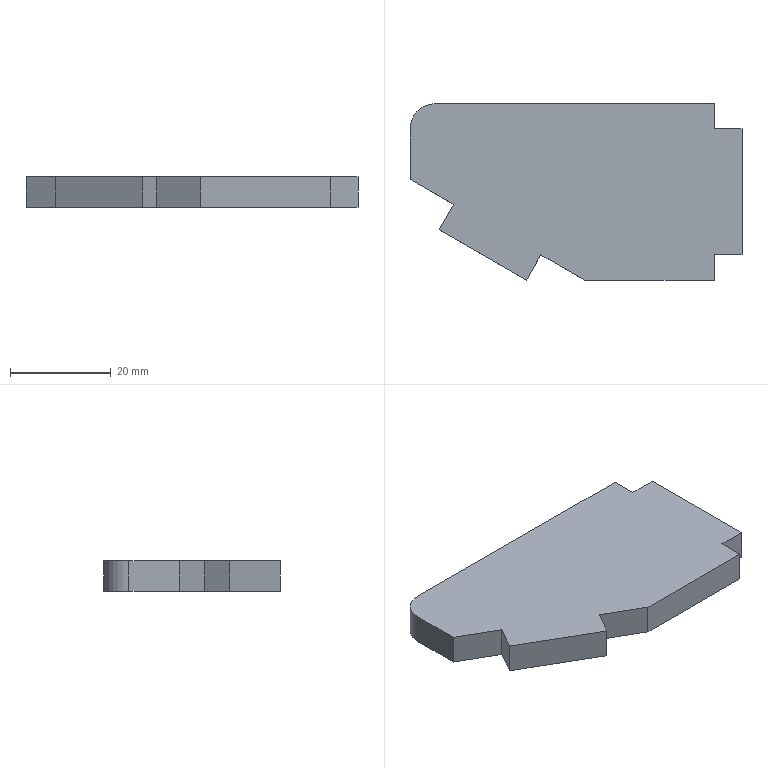Part | SolidWorks | features FlatPattern 1, SMBaseFlange 1, SheetMetal 1 | 1 solid | 16 faces | box 65.896 x 35.023 x 6 mm | volume 12093 mm3 | plane 15 | cylinder 1 | commonest cylinder face diameters 10 x1
STEP:
#1=CARTESIAN_POINT('',(-76.665,43.941,0.));
#2=VERTEX_POINT('',#1);
#3=CARTESIAN_POINT('',(-68.004,38.941,0.));
#4=VERTEX_POINT('',#3);
#5=CARTESIAN_POINT('',(-68.004,38.941,0.));
#6=DIRECTION('',(0.866,-0.5,0.));
#7=VECTOR('',#6,1000.);
#8=LINE('',#5,#7);
#9=EDGE_CURVE('',#2,#4,#8,.T.);
#10=ORIENTED_EDGE('',*,*,#9,.F.);
#11=CARTESIAN_POINT('',(-76.665,43.941,-6.));
#12=VERTEX_POINT('',#11);
#13=CARTESIAN_POINT('',(-76.665,43.941,-6.));
#14=DIRECTION('',(0.,0.,1.));
#15=VECTOR('',#14,1000.);
#16=LINE('',#13,#15);
#17=EDGE_CURVE('',#12,#2,#16,.T.);
#18=ORIENTED_EDGE('',*,*,#17,.F.);
#19=CARTESIAN_POINT('',(-68.004,38.941,-6.));
#20=VERTEX_POINT('',#19);
#21=CARTESIAN_POINT('',(-68.004,38.941,-6.));
#22=DIRECTION('',(0.866,-0.5,0.));
#23=VECTOR('',#22,1000.);
#24=LINE('',#21,#23);
#25=EDGE_CURVE('',#12,#20,#24,.T.);
#26=ORIENTED_EDGE('',*,*,#25,.T.);
#27=CARTESIAN_POINT('',(-68.004,38.941,-6.));
#28=DIRECTION('',(0.,0.,1.));
#29=VECTOR('',#28,1000.);
#30=LINE('',#27,#29);
#31=EDGE_CURVE('',#20,#4,#30,.T.);
#32=ORIENTED_EDGE('',*,*,#31,.T.);
#33=EDGE_LOOP('',(#10,#18,#26,#32));
#34=FACE_OUTER_BOUND('',#33,.T.);
#35=CARTESIAN_POINT('',(-68.004,38.941,-6.));
#36=DIRECTION('',(-0.5,-0.866,0.));
#37=DIRECTION('',(0.866,-0.5,0.));
#38=AXIS2_PLACEMENT_3D('',#35,#36,#37);
#39=PLANE('',#38);
#40=ADVANCED_FACE('',(#34),#39,.T.);
#41=CARTESIAN_POINT('',(-79.565,38.918,0.));
#42=VERTEX_POINT('',#41);
#43=CARTESIAN_POINT('',(-79.565,38.918,0.));
#44=DIRECTION('',(0.5,0.866,0.));
#45=VECTOR('',#44,1000.);
#46=LINE('',#43,#45);
#47=EDGE_CURVE('',#42,#2,#46,.T.);
#48=ORIENTED_EDGE('',*,*,#47,.F.);
#49=CARTESIAN_POINT('',(-79.565,38.918,-6.));
#50=VERTEX_POINT('',#49);
#51=CARTESIAN_POINT('',(-79.565,38.918,-6.));
#52=DIRECTION('',(0.,0.,1.));
#53=VECTOR('',#52,1000.);
#54=LINE('',#51,#53);
#55=EDGE_CURVE('',#50,#42,#54,.T.);
#56=ORIENTED_EDGE('',*,*,#55,.F.);
#57=CARTESIAN_POINT('',(-79.565,38.918,-6.));
#58=DIRECTION('',(0.5,0.866,0.));
#59=VECTOR('',#58,1000.);
#60=LINE('',#57,#59);
#61=EDGE_CURVE('',#50,#12,#60,.T.);
#62=ORIENTED_EDGE('',*,*,#61,.T.);
#63=ORIENTED_EDGE('',*,*,#17,.T.);
#64=EDGE_LOOP('',(#48,#56,#62,#63));
#65=FACE_OUTER_BOUND('',#64,.T.);
#66=CARTESIAN_POINT('',(-79.565,38.918,-6.));
#67=DIRECTION('',(0.866,-0.5,0.));
#68=DIRECTION('',(0.5,0.866,0.));
#69=AXIS2_PLACEMENT_3D('',#66,#67,#68);
#70=PLANE('',#69);
#71=ADVANCED_FACE('',(#65),#70,.T.);
#72=CARTESIAN_POINT('',(-96.885,48.918,0.));
#73=VERTEX_POINT('',#72);
#74=CARTESIAN_POINT('',(-96.885,48.918,0.));
#75=DIRECTION('',(0.866,-0.5,0.));
#76=VECTOR('',#75,1000.);
#77=LINE('',#74,#76);
#78=EDGE_CURVE('',#73,#42,#77,.T.);
#79=ORIENTED_EDGE('',*,*,#78,.F.);
#80=CARTESIAN_POINT('',(-96.885,48.918,-6.));
#81=VERTEX_POINT('',#80);
#82=CARTESIAN_POINT('',(-96.885,48.918,-6.));
#83=DIRECTION('',(0.,0.,1.));
#84=VECTOR('',#83,1000.);
#85=LINE('',#82,#84);
#86=EDGE_CURVE('',#81,#73,#85,.T.);
#87=ORIENTED_EDGE('',*,*,#86,.F.);
#88=CARTESIAN_POINT('',(-96.885,48.918,-6.));
#89=DIRECTION('',(0.866,-0.5,0.));
#90=VECTOR('',#89,1000.);
#91=LINE('',#88,#90);
#92=EDGE_CURVE('',#81,#50,#91,.T.);
#93=ORIENTED_EDGE('',*,*,#92,.T.);
#94=ORIENTED_EDGE('',*,*,#55,.T.);
#95=EDGE_LOOP('',(#79,#87,#93,#94));
#96=FACE_OUTER_BOUND('',#95,.T.);
#97=CARTESIAN_POINT('',(-96.885,48.918,-6.));
#98=DIRECTION('',(-0.5,-0.866,0.));
#99=DIRECTION('',(0.866,-0.5,0.));
#100=AXIS2_PLACEMENT_3D('',#97,#98,#99);
#101=PLANE('',#100);
#102=ADVANCED_FACE('',(#96),#101,.T.);
#103=CARTESIAN_POINT('',(-93.985,53.941,0.));
#104=VERTEX_POINT('',#103);
#105=CARTESIAN_POINT('',(-93.985,53.941,0.));
#106=DIRECTION('',(-0.5,-0.866,0.));
#107=VECTOR('',#106,1000.);
#108=LINE('',#105,#107);
#109=EDGE_CURVE('',#104,#73,#108,.T.);
#110=ORIENTED_EDGE('',*,*,#109,.F.);
#111=CARTESIAN_POINT('',(-93.985,53.941,-6.));
#112=VERTEX_POINT('',#111);
#113=CARTESIAN_POINT('',(-93.985,53.941,-6.));
#114=DIRECTION('',(0.,0.,1.));
#115=VECTOR('',#114,1000.);
#116=LINE('',#113,#115);
#117=EDGE_CURVE('',#112,#104,#116,.T.);
#118=ORIENTED_EDGE('',*,*,#117,.F.);
#119=CARTESIAN_POINT('',(-93.985,53.941,-6.));
#120=DIRECTION('',(-0.5,-0.866,0.));
#121=VECTOR('',#120,1000.);
#122=LINE('',#119,#121);
#123=EDGE_CURVE('',#112,#81,#122,.T.);
#124=ORIENTED_EDGE('',*,*,#123,.T.);
#125=ORIENTED_EDGE('',*,*,#86,.T.);
#126=EDGE_LOOP('',(#110,#118,#124,#125));
#127=FACE_OUTER_BOUND('',#126,.T.);
#128=CARTESIAN_POINT('',(-93.985,53.941,-6.));
#129=DIRECTION('',(-0.866,0.5,0.));
#130=DIRECTION('',(-0.5,-0.866,0.));
#131=AXIS2_PLACEMENT_3D('',#128,#129,#130);
#132=PLANE('',#131);
#133=ADVANCED_FACE('',(#127),#132,.T.);
#134=CARTESIAN_POINT('',(-102.646,58.941,0.));
#135=VERTEX_POINT('',#134);
#136=CARTESIAN_POINT('',(-93.985,53.941,0.));
#137=DIRECTION('',(0.866,-0.5,0.));
#138=VECTOR('',#137,1000.);
#139=LINE('',#136,#138);
#140=EDGE_CURVE('',#135,#104,#139,.T.);
#141=ORIENTED_EDGE('',*,*,#140,.F.);
#142=CARTESIAN_POINT('',(-102.646,58.941,-6.));
#143=VERTEX_POINT('',#142);
#144=CARTESIAN_POINT('',(-102.646,58.941,-6.));
#145=DIRECTION('',(0.,0.,1.));
#146=VECTOR('',#145,1000.);
#147=LINE('',#144,#146);
#148=EDGE_CURVE('',#143,#135,#147,.T.);
#149=ORIENTED_EDGE('',*,*,#148,.F.);
#150=CARTESIAN_POINT('',(-93.985,53.941,-6.));
#151=DIRECTION('',(0.866,-0.5,0.));
#152=VECTOR('',#151,1000.);
#153=LINE('',#150,#152);
#154=EDGE_CURVE('',#143,#112,#153,.T.);
#155=ORIENTED_EDGE('',*,*,#154,.T.);
#156=ORIENTED_EDGE('',*,*,#117,.T.);
#157=EDGE_LOOP('',(#141,#149,#155,#156));
#158=FACE_OUTER_BOUND('',#157,.T.);
#159=CARTESIAN_POINT('',(-93.985,53.941,-6.));
#160=DIRECTION('',(-0.5,-0.866,0.));
#161=DIRECTION('',(0.866,-0.5,0.));
#162=AXIS2_PLACEMENT_3D('',#159,#160,#161);
#163=PLANE('',#162);
#164=ADVANCED_FACE('',(#158),#163,.T.);
#165=CARTESIAN_POINT('',(-102.646,68.941,0.));
#166=VERTEX_POINT('',#165);
#167=CARTESIAN_POINT('',(-102.646,68.941,0.));
#168=DIRECTION('',(0.,-1.,0.));
#169=VECTOR('',#168,1000.);
#170=LINE('',#167,#169);
#171=EDGE_CURVE('',#166,#135,#170,.T.);
#172=ORIENTED_EDGE('',*,*,#171,.F.);
#173=CARTESIAN_POINT('',(-102.646,68.941,-6.));
#174=VERTEX_POINT('',#173);
#175=CARTESIAN_POINT('',(-102.646,68.941,-6.));
#176=DIRECTION('',(0.,0.,1.));
#177=VECTOR('',#176,1000.);
#178=LINE('',#175,#177);
#179=EDGE_CURVE('',#174,#166,#178,.T.);
#180=ORIENTED_EDGE('',*,*,#179,.F.);
#181=CARTESIAN_POINT('',(-102.646,68.941,-6.));
#182=DIRECTION('',(0.,-1.,0.));
#183=VECTOR('',#182,1000.);
#184=LINE('',#181,#183);
#185=EDGE_CURVE('',#174,#143,#184,.T.);
#186=ORIENTED_EDGE('',*,*,#185,.T.);
#187=ORIENTED_EDGE('',*,*,#148,.T.);
#188=EDGE_LOOP('',(#172,#180,#186,#187));
#189=FACE_OUTER_BOUND('',#188,.T.);
#190=CARTESIAN_POINT('',(-102.646,68.941,-6.));
#191=DIRECTION('',(-1.,0.,0.));
#192=DIRECTION('',(0.,0.,1.));
#193=AXIS2_PLACEMENT_3D('',#190,#191,#192);
#194=PLANE('',#193);
#195=ADVANCED_FACE('',(#189),#194,.T.);
#196=CARTESIAN_POINT('',(-97.646,73.941,0.));
#197=VERTEX_POINT('',#196);
#198=CARTESIAN_POINT('',(-97.646,68.941,0.));
#199=DIRECTION('',(0.,0.,1.));
#200=DIRECTION('',(1.,0.,0.));
#201=AXIS2_PLACEMENT_3D('',#198,#199,#200);
#202=CIRCLE('',#201,5.);
#203=EDGE_CURVE('',#197,#166,#202,.T.);
#204=ORIENTED_EDGE('',*,*,#203,.F.);
#205=CARTESIAN_POINT('',(-97.646,73.941,-6.));
#206=VERTEX_POINT('',#205);
#207=CARTESIAN_POINT('',(-97.646,73.941,-6.));
#208=DIRECTION('',(0.,0.,1.));
#209=VECTOR('',#208,1000.);
#210=LINE('',#207,#209);
#211=EDGE_CURVE('',#206,#197,#210,.T.);
#212=ORIENTED_EDGE('',*,*,#211,.F.);
#213=CARTESIAN_POINT('',(-97.646,68.941,-6.));
#214=DIRECTION('',(0.,0.,1.));
#215=DIRECTION('',(1.,0.,0.));
#216=AXIS2_PLACEMENT_3D('',#213,#214,#215);
#217=CIRCLE('',#216,5.);
#218=EDGE_CURVE('',#206,#174,#217,.T.);
#219=ORIENTED_EDGE('',*,*,#218,.T.);
#220=ORIENTED_EDGE('',*,*,#179,.T.);
#221=EDGE_LOOP('',(#204,#212,#219,#220));
#222=FACE_OUTER_BOUND('',#221,.T.);
#223=CARTESIAN_POINT('',(-97.646,68.941,-6.));
#224=DIRECTION('',(0.,0.,1.));
#225=DIRECTION('',(1.,0.,0.));
#226=AXIS2_PLACEMENT_3D('',#223,#224,#225);
#227=CYLINDRICAL_SURFACE('',#226,5.);
#228=ADVANCED_FACE('',(#222),#227,.T.);
#229=CARTESIAN_POINT('',(-42.25,73.941,0.));
#230=VERTEX_POINT('',#229);
#231=CARTESIAN_POINT('',(-42.25,73.941,0.));
#232=DIRECTION('',(-1.,0.,0.));
#233=VECTOR('',#232,1000.);
#234=LINE('',#231,#233);
#235=EDGE_CURVE('',#230,#197,#234,.T.);
#236=ORIENTED_EDGE('',*,*,#235,.F.);
#237=CARTESIAN_POINT('',(-42.25,73.941,-6.));
#238=VERTEX_POINT('',#237);
#239=CARTESIAN_POINT('',(-42.25,73.941,-6.));
#240=DIRECTION('',(0.,0.,1.));
#241=VECTOR('',#240,1000.);
#242=LINE('',#239,#241);
#243=EDGE_CURVE('',#238,#230,#242,.T.);
#244=ORIENTED_EDGE('',*,*,#243,.F.);
#245=CARTESIAN_POINT('',(-42.25,73.941,-6.));
#246=DIRECTION('',(-1.,0.,0.));
#247=VECTOR('',#246,1000.);
#248=LINE('',#245,#247);
#249=EDGE_CURVE('',#238,#206,#248,.T.);
#250=ORIENTED_EDGE('',*,*,#249,.T.);
#251=ORIENTED_EDGE('',*,*,#211,.T.);
#252=EDGE_LOOP('',(#236,#244,#250,#251));
#253=FACE_OUTER_BOUND('',#252,.T.);
#254=CARTESIAN_POINT('',(-42.25,73.941,-6.));
#255=DIRECTION('',(0.,1.,0.));
#256=DIRECTION('',(-1.,0.,0.));
#257=AXIS2_PLACEMENT_3D('',#254,#255,#256);
#258=PLANE('',#257);
#259=ADVANCED_FACE('',(#253),#258,.T.);
#260=CARTESIAN_POINT('',(-42.25,68.941,0.));
#261=VERTEX_POINT('',#260);
#262=CARTESIAN_POINT('',(-42.25,68.941,0.));
#263=DIRECTION('',(0.,1.,0.));
#264=VECTOR('',#263,1000.);
#265=LINE('',#262,#264);
#266=EDGE_CURVE('',#261,#230,#265,.T.);
#267=ORIENTED_EDGE('',*,*,#266,.F.);
#268=CARTESIAN_POINT('',(-42.25,68.941,-6.));
#269=VERTEX_POINT('',#268);
#270=CARTESIAN_POINT('',(-42.25,68.941,-6.));
#271=DIRECTION('',(0.,0.,1.));
#272=VECTOR('',#271,1000.);
#273=LINE('',#270,#272);
#274=EDGE_CURVE('',#269,#261,#273,.T.);
#275=ORIENTED_EDGE('',*,*,#274,.F.);
#276=CARTESIAN_POINT('',(-42.25,68.941,-6.));
#277=DIRECTION('',(0.,1.,0.));
#278=VECTOR('',#277,1000.);
#279=LINE('',#276,#278);
#280=EDGE_CURVE('',#269,#238,#279,.T.);
#281=ORIENTED_EDGE('',*,*,#280,.T.);
#282=ORIENTED_EDGE('',*,*,#243,.T.);
#283=EDGE_LOOP('',(#267,#275,#281,#282));
#284=FACE_OUTER_BOUND('',#283,.T.);
#285=CARTESIAN_POINT('',(-42.25,68.941,-6.));
#286=DIRECTION('',(1.,0.,0.));
#287=DIRECTION('',(0.,1.,0.));
#288=AXIS2_PLACEMENT_3D('',#285,#286,#287);
#289=PLANE('',#288);
#290=ADVANCED_FACE('',(#284),#289,.T.);
#291=CARTESIAN_POINT('',(-36.75,68.941,0.));
#292=VERTEX_POINT('',#291);
#293=CARTESIAN_POINT('',(-36.75,68.941,0.));
#294=DIRECTION('',(-1.,0.,0.));
#295=VECTOR('',#294,1000.);
#296=LINE('',#293,#295);
#297=EDGE_CURVE('',#292,#261,#296,.T.);
#298=ORIENTED_EDGE('',*,*,#297,.F.);
#299=CARTESIAN_POINT('',(-36.75,68.941,-6.));
#300=VERTEX_POINT('',#299);
#301=CARTESIAN_POINT('',(-36.75,68.941,-6.));
#302=DIRECTION('',(0.,0.,1.));
#303=VECTOR('',#302,1000.);
#304=LINE('',#301,#303);
#305=EDGE_CURVE('',#300,#292,#304,.T.);
#306=ORIENTED_EDGE('',*,*,#305,.F.);
#307=CARTESIAN_POINT('',(-36.75,68.941,-6.));
#308=DIRECTION('',(-1.,0.,0.));
#309=VECTOR('',#308,1000.);
#310=LINE('',#307,#309);
#311=EDGE_CURVE('',#300,#269,#310,.T.);
#312=ORIENTED_EDGE('',*,*,#311,.T.);
#313=ORIENTED_EDGE('',*,*,#274,.T.);
#314=EDGE_LOOP('',(#298,#306,#312,#313));
#315=FACE_OUTER_BOUND('',#314,.T.);
#316=CARTESIAN_POINT('',(-36.75,68.941,-6.));
#317=DIRECTION('',(0.,1.,0.));
#318=DIRECTION('',(-1.,0.,0.));
#319=AXIS2_PLACEMENT_3D('',#316,#317,#318);
#320=PLANE('',#319);
#321=ADVANCED_FACE('',(#315),#320,.T.);
#322=CARTESIAN_POINT('',(-36.75,43.941,0.));
#323=VERTEX_POINT('',#322);
#324=CARTESIAN_POINT('',(-36.75,43.941,0.));
#325=DIRECTION('',(0.,1.,0.));
#326=VECTOR('',#325,1000.);
#327=LINE('',#324,#326);
#328=EDGE_CURVE('',#323,#292,#327,.T.);
#329=ORIENTED_EDGE('',*,*,#328,.F.);
#330=CARTESIAN_POINT('',(-36.75,43.941,-6.));
#331=VERTEX_POINT('',#330);
#332=CARTESIAN_POINT('',(-36.75,43.941,-6.));
#333=DIRECTION('',(0.,0.,1.));
#334=VECTOR('',#333,1000.);
#335=LINE('',#332,#334);
#336=EDGE_CURVE('',#331,#323,#335,.T.);
#337=ORIENTED_EDGE('',*,*,#336,.F.);
#338=CARTESIAN_POINT('',(-36.75,43.941,-6.));
#339=DIRECTION('',(0.,1.,0.));
#340=VECTOR('',#339,1000.);
#341=LINE('',#338,#340);
#342=EDGE_CURVE('',#331,#300,#341,.T.);
#343=ORIENTED_EDGE('',*,*,#342,.T.);
#344=ORIENTED_EDGE('',*,*,#305,.T.);
#345=EDGE_LOOP('',(#329,#337,#343,#344));
#346=FACE_OUTER_BOUND('',#345,.T.);
#347=CARTESIAN_POINT('',(-36.75,43.941,-6.));
#348=DIRECTION('',(1.,0.,0.));
#349=DIRECTION('',(0.,0.,-1.));
#350=AXIS2_PLACEMENT_3D('',#347,#348,#349);
#351=PLANE('',#350);
#352=ADVANCED_FACE('',(#346),#351,.T.);
#353=CARTESIAN_POINT('',(-42.25,43.941,0.));
#354=VERTEX_POINT('',#353);
#355=CARTESIAN_POINT('',(-42.25,43.941,0.));
#356=DIRECTION('',(1.,0.,0.));
#357=VECTOR('',#356,1000.);
#358=LINE('',#355,#357);
#359=EDGE_CURVE('',#354,#323,#358,.T.);
#360=ORIENTED_EDGE('',*,*,#359,.F.);
#361=CARTESIAN_POINT('',(-42.25,43.941,-6.));
#362=VERTEX_POINT('',#361);
#363=CARTESIAN_POINT('',(-42.25,43.941,-6.));
#364=DIRECTION('',(0.,0.,1.));
#365=VECTOR('',#364,1000.);
#366=LINE('',#363,#365);
#367=EDGE_CURVE('',#362,#354,#366,.T.);
#368=ORIENTED_EDGE('',*,*,#367,.F.);
#369=CARTESIAN_POINT('',(-42.25,43.941,-6.));
#370=DIRECTION('',(1.,0.,0.));
#371=VECTOR('',#370,1000.);
#372=LINE('',#369,#371);
#373=EDGE_CURVE('',#362,#331,#372,.T.);
#374=ORIENTED_EDGE('',*,*,#373,.T.);
#375=ORIENTED_EDGE('',*,*,#336,.T.);
#376=EDGE_LOOP('',(#360,#368,#374,#375));
#377=FACE_OUTER_BOUND('',#376,.T.);
#378=CARTESIAN_POINT('',(-42.25,43.941,-6.));
#379=DIRECTION('',(0.,-1.,0.));
#380=DIRECTION('',(0.,0.,-1.));
#381=AXIS2_PLACEMENT_3D('',#378,#379,#380);
#382=PLANE('',#381);
#383=ADVANCED_FACE('',(#377),#382,.T.);
#384=CARTESIAN_POINT('',(-42.25,38.941,0.));
#385=VERTEX_POINT('',#384);
#386=CARTESIAN_POINT('',(-42.25,38.941,0.));
#387=DIRECTION('',(0.,1.,0.));
#388=VECTOR('',#387,1000.);
#389=LINE('',#386,#388);
#390=EDGE_CURVE('',#385,#354,#389,.T.);
#391=ORIENTED_EDGE('',*,*,#390,.F.);
#392=CARTESIAN_POINT('',(-42.25,38.941,-6.));
#393=VERTEX_POINT('',#392);
#394=CARTESIAN_POINT('',(-42.25,38.941,-6.));
#395=DIRECTION('',(0.,0.,1.));
#396=VECTOR('',#395,1000.);
#397=LINE('',#394,#396);
#398=EDGE_CURVE('',#393,#385,#397,.T.);
#399=ORIENTED_EDGE('',*,*,#398,.F.);
#400=CARTESIAN_POINT('',(-42.25,38.941,-6.));
#401=DIRECTION('',(0.,1.,0.));
#402=VECTOR('',#401,1000.);
#403=LINE('',#400,#402);
#404=EDGE_CURVE('',#393,#362,#403,.T.);
#405=ORIENTED_EDGE('',*,*,#404,.T.);
#406=ORIENTED_EDGE('',*,*,#367,.T.);
#407=EDGE_LOOP('',(#391,#399,#405,#406));
#408=FACE_OUTER_BOUND('',#407,.T.);
#409=CARTESIAN_POINT('',(-42.25,38.941,-6.));
#410=DIRECTION('',(1.,0.,0.));
#411=DIRECTION('',(0.,0.,-1.));
#412=AXIS2_PLACEMENT_3D('',#409,#410,#411);
#413=PLANE('',#412);
#414=ADVANCED_FACE('',(#408),#413,.T.);
#415=CARTESIAN_POINT('',(-68.004,38.941,0.));
#416=DIRECTION('',(1.,0.,0.));
#417=VECTOR('',#416,1000.);
#418=LINE('',#415,#417);
#419=EDGE_CURVE('',#4,#385,#418,.T.);
#420=ORIENTED_EDGE('',*,*,#419,.F.);
#421=ORIENTED_EDGE('',*,*,#31,.F.);
#422=CARTESIAN_POINT('',(-68.004,38.941,-6.));
#423=DIRECTION('',(1.,0.,0.));
#424=VECTOR('',#423,1000.);
#425=LINE('',#422,#424);
#426=EDGE_CURVE('',#20,#393,#425,.T.);
#427=ORIENTED_EDGE('',*,*,#426,.T.);
#428=ORIENTED_EDGE('',*,*,#398,.T.);
#429=EDGE_LOOP('',(#420,#421,#427,#428));
#430=FACE_OUTER_BOUND('',#429,.T.);
#431=CARTESIAN_POINT('',(-68.004,38.941,-6.));
#432=DIRECTION('',(0.,-1.,0.));
#433=DIRECTION('',(0.,0.,-1.));
#434=AXIS2_PLACEMENT_3D('',#431,#432,#433);
#435=PLANE('',#434);
#436=ADVANCED_FACE('',(#430),#435,.T.);
#437=ORIENTED_EDGE('',*,*,#25,.F.);
#438=ORIENTED_EDGE('',*,*,#61,.F.);
#439=ORIENTED_EDGE('',*,*,#92,.F.);
#440=ORIENTED_EDGE('',*,*,#123,.F.);
#441=ORIENTED_EDGE('',*,*,#154,.F.);
#442=ORIENTED_EDGE('',*,*,#185,.F.);
#443=ORIENTED_EDGE('',*,*,#218,.F.);
#444=ORIENTED_EDGE('',*,*,#249,.F.);
#445=ORIENTED_EDGE('',*,*,#280,.F.);
#446=ORIENTED_EDGE('',*,*,#311,.F.);
#447=ORIENTED_EDGE('',*,*,#342,.F.);
#448=ORIENTED_EDGE('',*,*,#373,.F.);
#449=ORIENTED_EDGE('',*,*,#404,.F.);
#450=ORIENTED_EDGE('',*,*,#426,.F.);
#451=EDGE_LOOP('',(#437,#438,#439,#440,#441,#442,#443,#444,#445,#446,#447,#448,#449,#450));
#452=FACE_OUTER_BOUND('',#451,.T.);
#453=CARTESIAN_POINT('',(-97.646,68.941,-6.));
#454=DIRECTION('',(0.,0.,1.));
#455=DIRECTION('',(1.,0.,0.));
#456=AXIS2_PLACEMENT_3D('',#453,#454,#455);
#457=PLANE('',#456);
#458=ADVANCED_FACE('',(#452),#457,.F.);
#459=ORIENTED_EDGE('',*,*,#9,.T.);
#460=ORIENTED_EDGE('',*,*,#419,.T.);
#461=ORIENTED_EDGE('',*,*,#390,.T.);
#462=ORIENTED_EDGE('',*,*,#359,.T.);
#463=ORIENTED_EDGE('',*,*,#328,.T.);
#464=ORIENTED_EDGE('',*,*,#297,.T.);
#465=ORIENTED_EDGE('',*,*,#266,.T.);
#466=ORIENTED_EDGE('',*,*,#235,.T.);
#467=ORIENTED_EDGE('',*,*,#203,.T.);
#468=ORIENTED_EDGE('',*,*,#171,.T.);
#469=ORIENTED_EDGE('',*,*,#140,.T.);
#470=ORIENTED_EDGE('',*,*,#109,.T.);
#471=ORIENTED_EDGE('',*,*,#78,.T.);
#472=ORIENTED_EDGE('',*,*,#47,.T.);
#473=EDGE_LOOP('',(#459,#460,#461,#462,#463,#464,#465,#466,#467,#468,#469,#470,#471,#472));
#474=FACE_OUTER_BOUND('',#473,.T.);
#475=CARTESIAN_POINT('',(-97.646,68.941,0.));
#476=DIRECTION('',(0.,0.,1.));
#477=DIRECTION('',(1.,0.,0.));
#478=AXIS2_PLACEMENT_3D('',#475,#476,#477);
#479=PLANE('',#478);
#480=ADVANCED_FACE('',(#474),#479,.T.);
#481=CLOSED_SHELL('',(#40,#71,#102,#133,#164,#195,#228,#259,#290,#321,#352,#383,#414,#436,#458,#480));
#482=MANIFOLD_SOLID_BREP('',#481);
#483=CARTESIAN_POINT('',(0.,0.,0.));
#484=DIRECTION('',(0.,0.,1.));
#485=DIRECTION('',(1.,0.,0.));
#486=AXIS2_PLACEMENT_3D('',#483,#484,#485);
#487=(LENGTH_UNIT()NAMED_UNIT(*)SI_UNIT(.MILLI.,.METRE.));
#488=UNCERTAINTY_MEASURE_WITH_UNIT(LENGTH_MEASURE(0.00001),#487,'','');
#489=(NAMED_UNIT(*)PLANE_ANGLE_UNIT()SI_UNIT($,.RADIAN.));
#490=(NAMED_UNIT(*)SI_UNIT($,.STERADIAN.)SOLID_ANGLE_UNIT());
#491=(GEOMETRIC_REPRESENTATION_CONTEXT(3)GLOBAL_UNCERTAINTY_ASSIGNED_CONTEXT((#488))GLOBAL_UNIT_ASSIGNED_CONTEXT((#487,#489,#490))REPRESENTATION_CONTEXT('',''));
#492=ADVANCED_BREP_SHAPE_REPRESENTATION('',(#482,#486),#491);